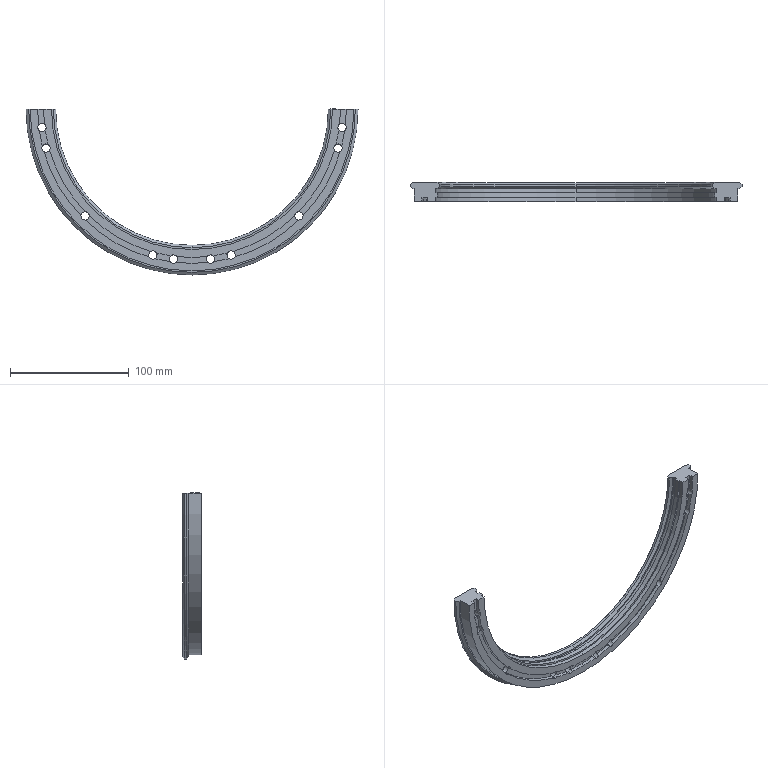Part | SolidWorks | features BaseBody 1 | 1 solid | 111 faces | box 280 x 16 x 140 mm | volume 112815 mm3 | cylinder 75 | plane 30 | cone 6 | commonest cylinder face diameters 7 x20 11 x20 250 x12 260 x12 237 x4 230 x2